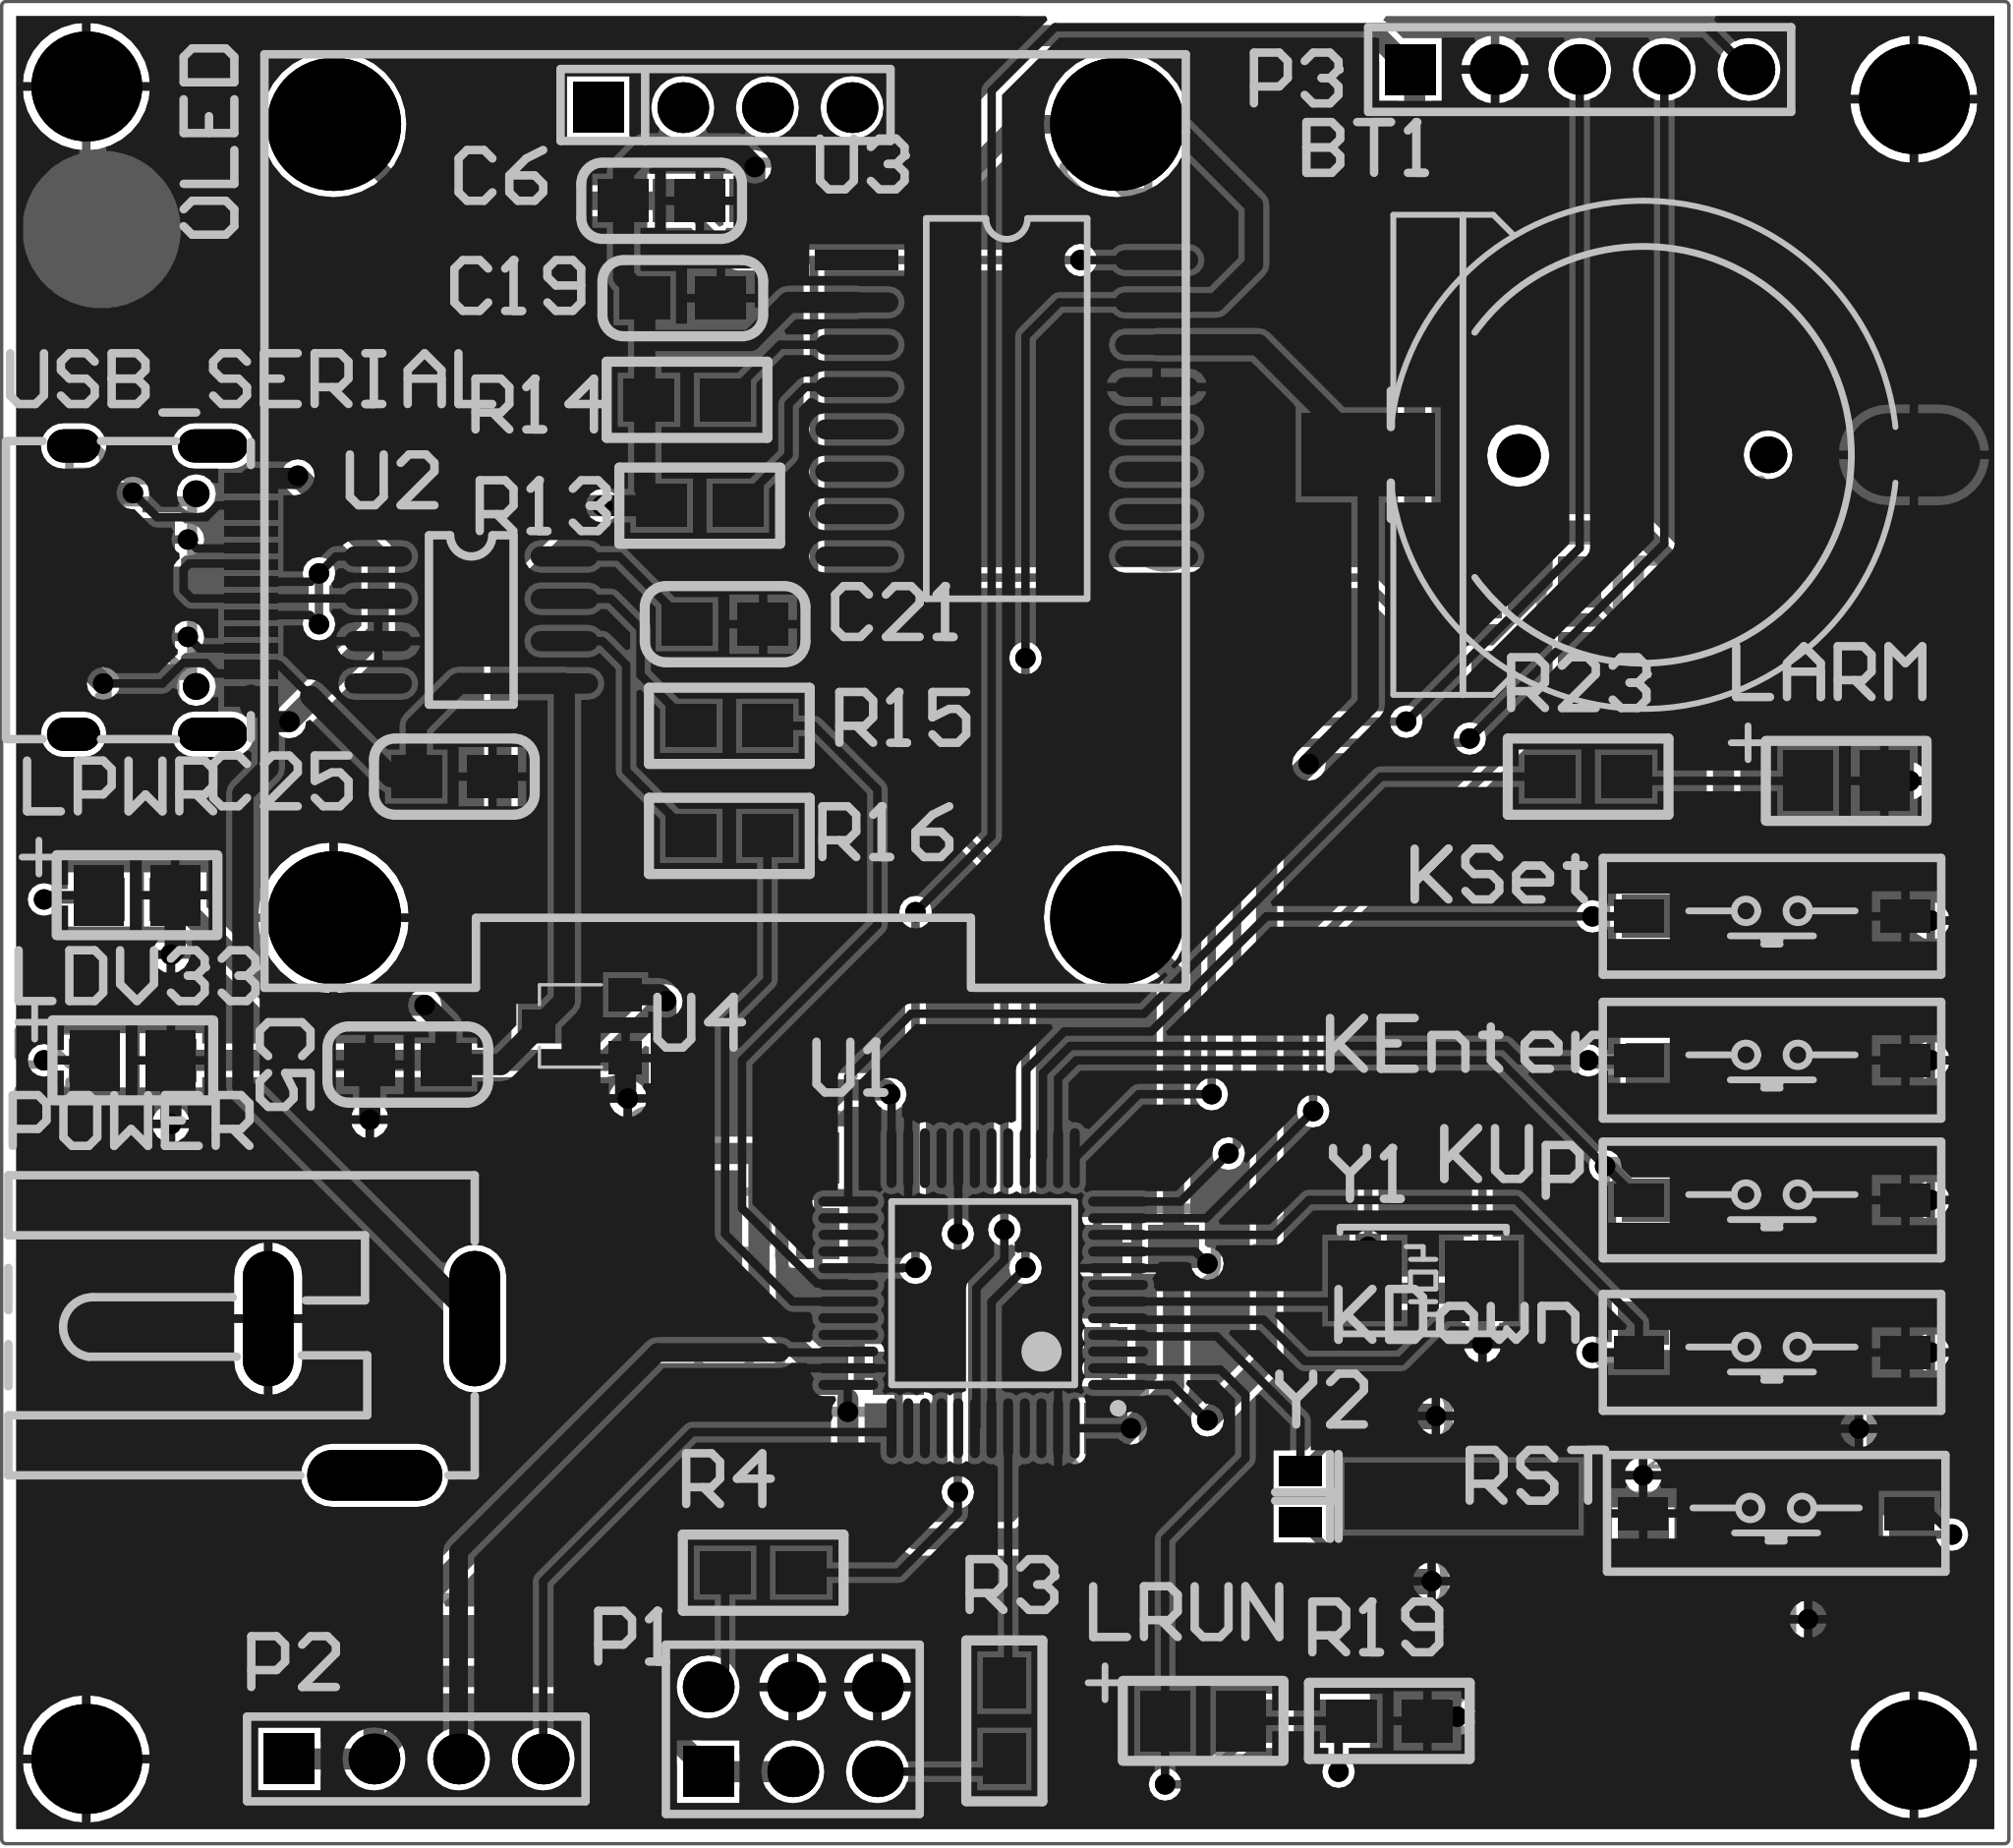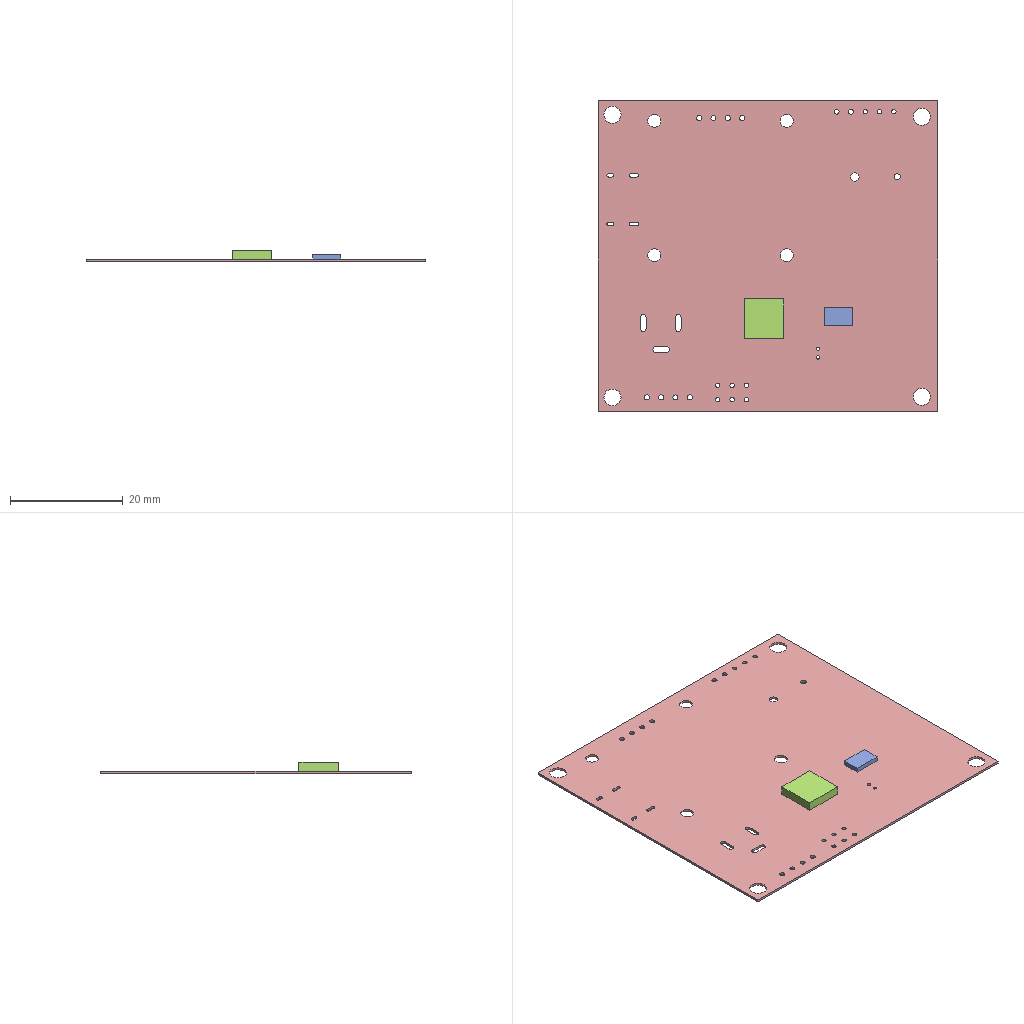Circuit board layout | Altium Designer | box 60.3 x 55.3 x 2 mm
Layer stack:
# Altium Designer layer stack of  (unit mm; dielectric type: 0 none, 1 core, 2 prepreg, 3 surface material)
index,name,kind,layer,copper_thickness_mm,dielectric_type,dielectric_thickness_mm,dielectric_material,dielectric_constant
0,Top Paste,other,,,,,,
1,Top Overlay,other,,,,,,
2,Top Solder,dielectric,,,3,0.0102,Solder Resist,3.5
3,Top Layer,copper,Top Layer,0.0356,,,,
4,Dielectric 1,dielectric,,,0,0.32,FR-4,4.8
5,Bottom Layer,copper,Bottom Layer,0.0356,,,,
6,Bottom Solder,dielectric,,,3,0.0102,Solder Resist,3.5
7,Bottom Overlay,other,,,,,,
8,Bottom Paste,other,,,,,,
# drill layer pairs: low layer,high layer
drill_pair,Top Layer,Bottom Layer
Part placement:
Designator,Comment,Layer,Footprint,Center-X(mm),Center-Y(mm),Rotation
Y2,32.768K,TopLayer,OSC_2*6,41.275,10.287,360
Y1,8MHZ,TopLayer,OSC_5032-2P,42.545,16.764,0
USB_SERIAL,type_C_16pins,TopLayer,TYPE_C_16PIN,4.692,37.472,90
U4,XC6206P332MR,TopLayer,SOT-23S,17.302,24.384,90
U3,DS3231SN,TopLayer,SOP-16,30.044,42.926,0
U2,CH340N,TopLayer,SO-8,13.97,36.576,0
U1,STM32F103C8T6A,TopLayer,LQFP48,29.337,16.383,180
T1,S8550,BottomLayer,SOT-23,43.434,36.132,270
RST,SW-PB,TopLayer,KEY_8mm,53.149,9.779,180
R23,Res2,TopLayer,R0805,47.498,31.877,180
R22,Res2,BottomLayer,R0805,42.545,21.717,360
R21,Res2,BottomLayer,R0805,21.336,49.149,360
R20,Res2,BottomLayer,R0805,26.924,49.149,180
R19,Res2,TopLayer,R0805,41.529,3.556,180
R18,Res2,BottomLayer,R0805,50.292,15.494,360
R17,Res2,BottomLayer,R0805,50.165,35.941,90
R16,Res2,TopLayer,R0805,21.717,30.099,360
R15,Res2,TopLayer,R0805,21.717,33.401,360
R14,Res2,TopLayer,R0805,20.447,43.18,180
R13,Res2,TopLayer,R0805,20.828,40.005,180
R12,Res2,BottomLayer,R0805,47.244,36.576,270
R11,Res2,BottomLayer,R0805,38.862,3.556,180
R10,Res2,BottomLayer,R0805,3.175,36.068,180
R9,Res2,BottomLayer,R0805,3.175,38.989,180
R8,Res2,BottomLayer,R0805,50.419,19.177,360
R7,Res2,BottomLayer,R0805,3.937,28.194,180
R6,Res2,BottomLayer,R0805,50.546,23.241,360
R5,Res2,BottomLayer,R0805,50.419,27.686,360
R4,Res2,TopLayer,R0805,22.733,8.001,360
R3,Res2,TopLayer,R0805,29.972,3.556,270
R2,Res2,BottomLayer,R0805,50.292,9.144,360
R1,Res2,BottomLayer,R0805,3.81,23.368,180
POWER,5.2/2.1,TopLayer,SWC_SET,10.974,13.271,360
P3,SIP5,TopLayer,HDR1X5,47.244,53.086,360
P2,SWD,TopLayer,HDR1X4,12.319,2.413,360
P1,IDC3*2,TopLayer,HDR2X3,23.622,3.302,360
OLED,OLED_IIC,TopLayer,OLED,21.59,39.793,0
LRUN,RLED,TopLayer,LED0805,35.941,3.556,360
LPWR,RLED,TopLayer,LED0805,3.937,28.321,360
LDV33,RLED,TopLayer,LED0805,3.81,23.368,360
LARM,RLED,TopLayer,LED0805,55.245,31.75,360
KUp,SW-PB,TopLayer,KEY_8mm,53.022,19.177,180
KSet,SW-PB,TopLayer,KEY_8mm,53.022,27.686,180
KEnter,SW-PB,TopLayer,KEY_8mm,53.022,23.368,180
KDown,SW-PB,TopLayer,KEY_8mm,53.022,14.605,180
D1,IN4148,BottomLayer,D0805,55.778,9.144,180
C24,104,BottomLayer,C0805,53.594,12.319,180
C21,104,TopLayer,C0805,21.59,36.449,360
C19,105,TopLayer,C0805,20.32,46.228,180
C14,22p,BottomLayer,C0603,40.894,17.081,180
C13,22p,BottomLayer,C0603,44.323,16.828,180
C12,10p,BottomLayer,C0603,41.719,12.7,270
C11,106,BottomLayer,C0805,43.434,50.038,180
C10,104,BottomLayer,C0805,24.384,19.304,90
C9,10p,BottomLayer,C0603,41.593,7.747,270
C7,104,BottomLayer,C0805,33.02,13.462,270
C6,106,TopLayer,C0805,19.685,49.149,180
C5,106,TopLayer,C0805,12.065,23.241,360
C4,104,BottomLayer,C0805,33.909,17.78,360
C3,104,BottomLayer,C0805,25.654,13.97,180
C2,105,BottomLayer,C0805,56.007,6.604,360
C1,104,BottomLayer,C0805,12.573,6.096,360
BT1,1220_3V,TopLayer,CR1220,49.086,41.517,180
BEEP,Bell,BottomLayer,HN9650B,31.649,36.195,90
Pad and via stacks:
# Altium Designer via and pad stacks of  (unit mm). Each distinct definition once, with the count of objects using it.
# via: kind,start_layer,end_layer,hole_mm,diameter_mm,mode(0 simple;1 top-mid-bottom;2 full stack),diameter_per_layer,count,example_net
# pad: kind,layer,hole_mm,hole_type(0 round;1 square;2 slot),plating,top_size,top_shape(1 round;2 rect;3 octagon;9 rounded rect),mid_size,bottom_size,mode,footprint,size_per_layer,count,example
pad,Top Layer,0,0,plated,1.524x1.27,2,1.524x1.27,1.524x1.27,0,C0805,,10,C19.2
pad,Top Layer,0,0,plated,0.3x1.8,1,0.3x1.8,0.3x1.8,0,LQFP48,,48,U1.36
pad,Top Layer,0,0,plated,2.5x0.6,2,2.5x0.6,2.5x0.6,0,SOP-16,,1,U3.1
pad,Top Layer,0,0,plated,2.5x0.6,1,2.5x0.6,2.5x0.6,0,SOP-16,,15,U3.2
pad,Top Layer,0,0,plated,2.5x4,1,2.5x4,2.5x4,0,CR1220,,1,BT1.2
pad,Top Layer,0,0,plated,2.5x4,2,2.5x4,2.5x4,0,CR1220,,1,BT1.1
pad,Top Layer,0,0,plated,7x2,2,7x2,7x2,0,OSC_2*6,,1,Y2.0
pad,Top Layer,0,0,plated,1.524x1.27,2,1.524x1.27,1.524x1.27,0,R0805,,16,R23.2
pad,Top Layer,0,0,plated,1.5x1.8,2,1.5x1.8,1.5x1.8,0,LED0805,,8,LPWR.A
pad,Top Layer,0,0,unplated,2.4x2.2,2,2.4x2.2,2.4x2.2,0,OSC 5032-2P,,2,Y1.2
pad,Top Layer,0,0,plated,2.032x0.6096,1,2.032x0.6096,2.032x0.6096,0,SO-8,,8,U2.4
pad,Top Layer,0,0,plated,1x1,2,1x1,1x1,0,SOT-23S,,3,U4.1
pad,Top Layer,0,0,plated,0.31x1.6,2,0.31x1.6,0.31x1.6,0,TYPE_C_16PIN,,6,USB_SERIAL.A12
pad,Top Layer,0,0,plated,0.3x1.6,2,0.3x1.6,0.3x1.6,0,TYPE_C_16PIN,,10,USB_SERIAL.B8
pad,Top Layer,0,0,plated,1.5x1,2,1.5x1,1.5x1,0,KEY_8mm,,10,KSet.2
pad,Multi-Layer,1.5,0,unplated,1.3x1.3,1,1.3x1.3,1.3x1.3,0,CR1220,,1,BT1.0
pad,Multi-Layer,1.1,0,unplated,1.1x1.1,1,1.1x1.1,1.1x1.1,0,CR1220,,1,BT1.0
pad,Multi-Layer,1,2,plated,1.524x4.064,1,1.524x4.064,1.524x4.064,0,SWC_SET,,2,POWER.3
pad,Multi-Layer,1,2,plated,4.064x1.524,1,4.064x1.524,4.064x1.524,0,SWC_SET,,1,POWER.0
pad,Multi-Layer,0.6,0,plated,1.27x0.889,2,1.27x0.889,1.27x0.889,0,OSC_2*6,,2,Y2.1
pad,Multi-Layer,0.9,0,plated,1.524x1.524,1,1.524x1.524,1.524x1.524,0,HDR1X4,,3,P2.3
pad,Multi-Layer,0.9,0,plated,1.524x1.524,2,1.524x1.524,1.524x1.524,0,HDR1X4,,1,P2.1
pad,Multi-Layer,0.762,0,plated,1.524x1.524,1,1.524x1.524,1.524x1.524,0,HDR2X3,,5,P1.2
pad,Multi-Layer,0.762,0,plated,1.524x1.524,2,1.524x1.524,1.524x1.524,0,HDR2X3,,1,P1.1
pad,Multi-Layer,0.9,0,plated,1.524x1.524,1,1.524x1.524,1.524x1.524,0,OLED,,3,OLED.20
pad,Multi-Layer,0.9,0,plated,1.524x1.524,2,1.524x1.524,1.524x1.524,0,OLED,,1,OLED.17
pad,Multi-Layer,2.3,0,plated,4x4,1,4x4,4x4,0,OLED,,4,OLED.4
pad,Multi-Layer,0.6,2,plated,1x1.6,1,1x1.6,1x1.6,0,TYPE_C_16PIN,,2,USB_SERIAL.19
pad,Multi-Layer,0.6,2,plated,1x2.1,1,1x2.1,1x2.1,0,TYPE_C_16PIN,,2,USB_SERIAL.17
pad,Multi-Layer,0.9,0,plated,1.524x1.524,1,1.524x1.524,1.524x1.524,0,HDR1X5,,1,P3.2
pad,Multi-Layer,0.9,0,plated,1.524x1.524,2,1.524x1.524,1.524x1.524,0,HDR1X5,,1,P3.1
pad,Multi-Layer,0.762,0,plated,1.524x1.524,1,1.524x1.524,1.524x1.524,0,HDR1X5,,3,P3.3
pad,Multi-Layer,3.048,0,plated,3.302x3.302,1,3.302x3.302,3.302x3.302,0,,,4,2
pad,Bottom Layer,0,0,plated,1.524x1.27,2,1.524x1.27,1.524x1.27,0,R0805,,30,R20.2
pad,Bottom Layer,0,0,plated,1.524x1.27,2,1.524x1.27,1.524x1.27,0,C0805,,18,C7.2
pad,Bottom Layer,0,0,plated,0.762x0.762,2,0.762x0.762,0.762x0.762,0,C0603,,8,C9.2
pad,Bottom Layer,0,0,plated,1.5x3.4,2,1.5x3.4,1.5x3.4,0,HN9650B,,2,BEEP.1
pad,Bottom Layer,0,0,plated,0.9144x1.27,2,0.9144x1.27,0.9144x1.27,0,SOT-23,,1,T1.3
pad,Bottom Layer,0,0,plated,0.9144x0.9144,2,0.9144x0.9144,0.9144x0.9144,0,SOT-23,,2,T1.2
pad,Bottom Layer,0,0,plated,1x0.8,2,1x0.8,1x0.8,0,D0805,,2,D1.A
via,Top Layer,Bottom Layer,0.8,0.8,0,,2,
via,Top Layer,Bottom Layer,0.3048,0.6096,0,,58,NetR10_1
Copper pours:
name,layer,net,type(0 solid;1 hatched;2 none)
G,Top Layer,GND,0
G,Bottom Layer,GND,0
Design rules, without the lines most boards share:
# Altium Designer design rules of  (exported by Altium Designer, unit mm)
# columns: name | kind | enabled | priority | scope1 | scope2 | descriptor | typed fields (field=value)
SilkToSilkClearance | 55 | enabled | 1 | All | All | Silk to Silk (Clearance=0mil) (All),(All) |
SilkToSolderMaskClearance | 54 | enabled | 1 | IsPad | All | Silk To Solder Mask (Clearance=0mil) (IsPad),(All) |
MinimumSolderMaskSliver | 53 | enabled | 1 | All | All | Minimum Solder Mask Sliver (Gap=0mil) (All),(All) |
HoleToHoleClearance | 52 | enabled | 1 | All | All | Hole To Hole Clearance (Gap=10mil) (All),(All) | gap=0.254
DiffPairsRouting | 51 | enabled | 1 | All | All | Differential Pairs Uncoupled Length using the Gap Constraints (Min=10mil) (Max=10mil) (Prefered=10mil)  and Width Constraints (Min=10mil) (Max=15mil) (Prefered=10mil) (All) |
SolderMaskExpansion | 13 | enabled | 1 | All | All | Solder Mask Expansion (Expansion =4mil) (All) | expansion=0.1016
PasteMaskExpansion | 14 | enabled | 1 | All | All | Paste Mask Expansion (Expansion =0mil) (All) | expansion=0
RoutingVias | 11 | enabled | 1 | All | All | Routing Via (MinHoleWidth=28mil) (MaxHoleWidth=28mil) (PreferredHoleWidth=28mil) (MinWidth=50mil) (MaxWidth=50mil) (PreferedWidth=50mil) (All) | via_min_hole=0.7112 via_max_hole=0.7112 via_preferred_diameter=1.27 via_preferred_hole=0.7112
Width | 2 | enabled | 1 | All | All | Width Constraint (Min=10mil) (Max=25mil) (Preferred=10mil) (All) |
PolygonConnect | 20 | enabled | 1 | All | All | Polygon Connect Rule(Relief Connect )(Conductor Width=10mil) (Relief Angle=90 Angle) (Entries=4) (Air Gap Width=10mil) (All),(All) | connect_style(0=relief,1=direct,2=none)=0 relief_conductor_width=0.254 relief_entries=4
PlaneConnect | 6 | enabled | 1 | All | All | Power Plane Connect Rule(Relief Connect )(Expansion=20mil) (Conductor Width=10mil) (Air Gap=10mil) (Entries=4) (All) | relief_conductor_width=0.254 relief_entries=4 relief_expansion=0.508
Clearance | 0 | enabled | 1 | All | All | Clearance Constraint (Gap=5mil) (All),(All) | gap=0.127